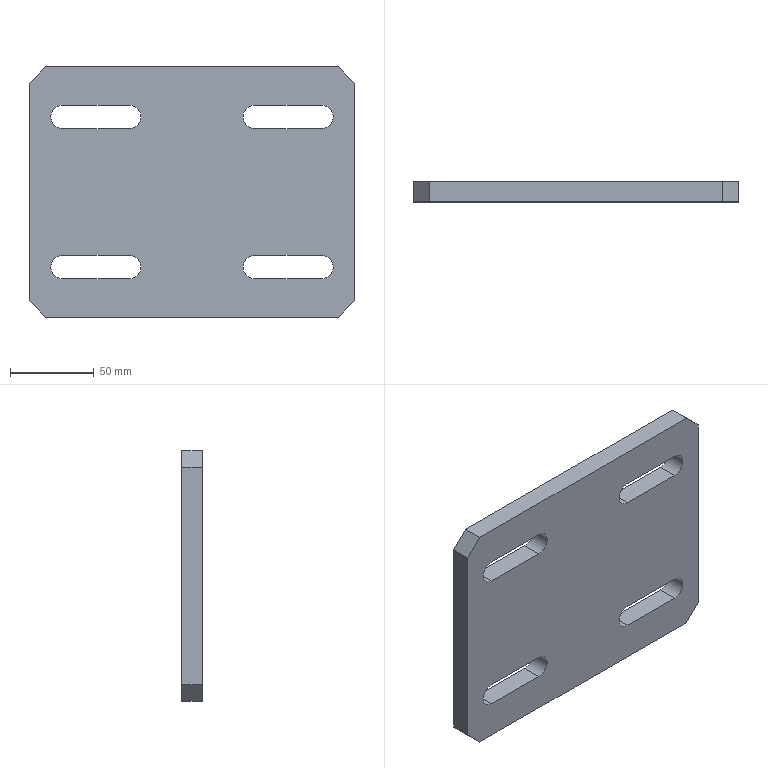Part | STEP file | E3-运输活动Plate 1 | 1 solid | 26 faces | box 195 x 12 x 150 mm | volume 314331 mm3 | plane 18 | cylinder 8 | commonest cylinder face diameters 14 x8